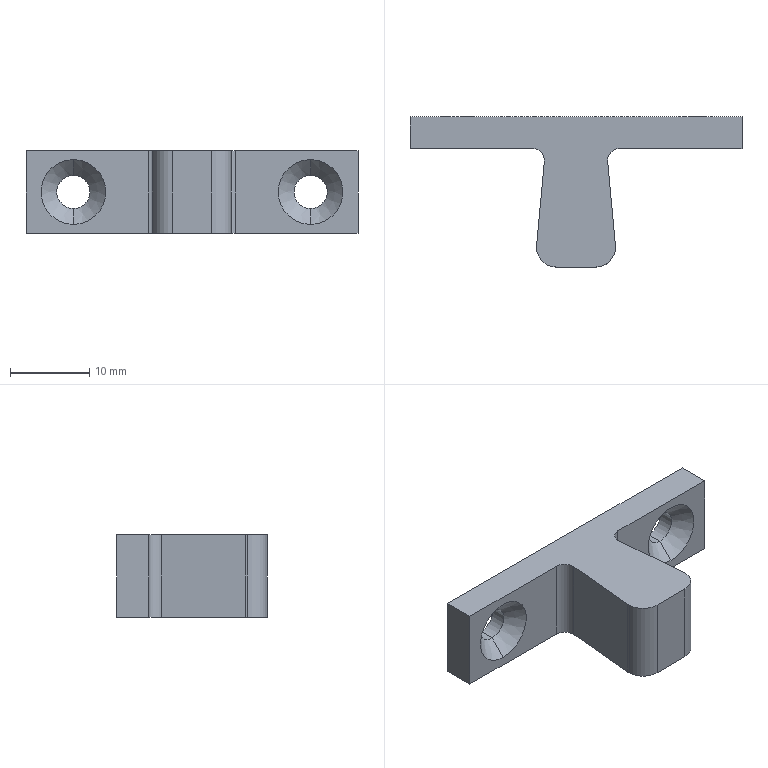Part | STEP file | CATCHE2_MISUMI_BCAS70_Latch | 1 solid | 24 faces | box 42 x 19 x 10.5 mm | volume 2994 mm3 | cylinder 10 | plane 10 | cone 4 | commonest cylinder face diameters 4.2 x4 3 x3 5 x3
STEP:
#1=CARTESIAN_POINT('',(-15.,-2.,2.1));
#2=VERTEX_POINT('',#1);
#3=CARTESIAN_POINT('',(-15.,-2.,-2.1));
#4=VERTEX_POINT('',#3);
#5=CARTESIAN_POINT('',(-15.,-2.,0.));
#6=DIRECTION('',(0.,-1.,0.));
#7=DIRECTION('',(0.,0.,-1.));
#8=AXIS2_PLACEMENT_3D('',#5,#6,#7);
#9=CIRCLE('',#8,2.1);
#10=EDGE_CURVE('',#2,#4,#9,.T.);
#11=ORIENTED_EDGE('',*,*,#10,.F.);
#12=CARTESIAN_POINT('',(-15.,-4.,4.1));
#13=VERTEX_POINT('',#12);
#14=CARTESIAN_POINT('',(-15.,-4.,4.1));
#15=DIRECTION('',(0.,-0.7071,0.7071));
#16=VECTOR('',#15,1000.);
#17=LINE('',#14,#16);
#18=EDGE_CURVE('',#2,#13,#17,.T.);
#19=ORIENTED_EDGE('',*,*,#18,.T.);
#20=CARTESIAN_POINT('',(-15.,-4.,-4.1));
#21=VERTEX_POINT('',#20);
#22=CARTESIAN_POINT('',(-15.,-4.,0.));
#23=DIRECTION('',(0.,-1.,0.));
#24=DIRECTION('',(0.,0.,-1.));
#25=AXIS2_PLACEMENT_3D('',#22,#23,#24);
#26=CIRCLE('',#25,4.1);
#27=EDGE_CURVE('',#13,#21,#26,.T.);
#28=ORIENTED_EDGE('',*,*,#27,.T.);
#29=CARTESIAN_POINT('',(-15.,-4.,-4.1));
#30=DIRECTION('',(0.,-0.7071,-0.7071));
#31=VECTOR('',#30,1000.);
#32=LINE('',#29,#31);
#33=EDGE_CURVE('',#4,#21,#32,.T.);
#34=ORIENTED_EDGE('',*,*,#33,.F.);
#35=EDGE_LOOP('',(#11,#19,#28,#34));
#36=FACE_OUTER_BOUND('',#35,.T.);
#37=CARTESIAN_POINT('',(-15.,-4.,0.));
#38=DIRECTION('',(0.,-1.,0.));
#39=DIRECTION('',(0.,0.,-1.));
#40=AXIS2_PLACEMENT_3D('',#37,#38,#39);
#41=CONICAL_SURFACE('',#40,4.1,0.7854);
#42=ADVANCED_FACE('',(#36),#41,.F.);
#43=CARTESIAN_POINT('',(-15.,0.,2.1));
#44=VERTEX_POINT('',#43);
#45=CARTESIAN_POINT('',(-15.,0.,-2.1));
#46=VERTEX_POINT('',#45);
#47=CARTESIAN_POINT('',(-15.,0.,0.));
#48=DIRECTION('',(0.,-1.,0.));
#49=DIRECTION('',(0.,0.,-1.));
#50=AXIS2_PLACEMENT_3D('',#47,#48,#49);
#51=CIRCLE('',#50,2.1);
#52=EDGE_CURVE('',#44,#46,#51,.T.);
#53=ORIENTED_EDGE('',*,*,#52,.F.);
#54=CARTESIAN_POINT('',(-15.,-4.,2.1));
#55=DIRECTION('',(0.,-1.,0.));
#56=VECTOR('',#55,1000.);
#57=LINE('',#54,#56);
#58=EDGE_CURVE('',#44,#2,#57,.T.);
#59=ORIENTED_EDGE('',*,*,#58,.T.);
#60=ORIENTED_EDGE('',*,*,#10,.T.);
#61=CARTESIAN_POINT('',(-15.,-4.,-2.1));
#62=DIRECTION('',(0.,-1.,0.));
#63=VECTOR('',#62,1000.);
#64=LINE('',#61,#63);
#65=EDGE_CURVE('',#46,#4,#64,.T.);
#66=ORIENTED_EDGE('',*,*,#65,.F.);
#67=EDGE_LOOP('',(#53,#59,#60,#66));
#68=FACE_OUTER_BOUND('',#67,.T.);
#69=CARTESIAN_POINT('',(-15.,-4.,0.));
#70=DIRECTION('',(0.,-1.,0.));
#71=DIRECTION('',(0.,0.,-1.));
#72=AXIS2_PLACEMENT_3D('',#69,#70,#71);
#73=CYLINDRICAL_SURFACE('',#72,2.1);
#74=ADVANCED_FACE('',(#68),#73,.F.);
#75=CARTESIAN_POINT('',(15.,-2.,2.1));
#76=VERTEX_POINT('',#75);
#77=CARTESIAN_POINT('',(15.,-2.,-2.1));
#78=VERTEX_POINT('',#77);
#79=CARTESIAN_POINT('',(15.,-2.,0.));
#80=DIRECTION('',(0.,-1.,0.));
#81=DIRECTION('',(0.,0.,-1.));
#82=AXIS2_PLACEMENT_3D('',#79,#80,#81);
#83=CIRCLE('',#82,2.1);
#84=EDGE_CURVE('',#76,#78,#83,.T.);
#85=ORIENTED_EDGE('',*,*,#84,.F.);
#86=CARTESIAN_POINT('',(15.,-4.,4.1));
#87=VERTEX_POINT('',#86);
#88=CARTESIAN_POINT('',(15.,-4.,4.1));
#89=DIRECTION('',(0.,-0.7071,0.7071));
#90=VECTOR('',#89,1000.);
#91=LINE('',#88,#90);
#92=EDGE_CURVE('',#76,#87,#91,.T.);
#93=ORIENTED_EDGE('',*,*,#92,.T.);
#94=CARTESIAN_POINT('',(15.,-4.,-4.1));
#95=VERTEX_POINT('',#94);
#96=CARTESIAN_POINT('',(15.,-4.,0.));
#97=DIRECTION('',(0.,-1.,0.));
#98=DIRECTION('',(0.,0.,-1.));
#99=AXIS2_PLACEMENT_3D('',#96,#97,#98);
#100=CIRCLE('',#99,4.1);
#101=EDGE_CURVE('',#87,#95,#100,.T.);
#102=ORIENTED_EDGE('',*,*,#101,.T.);
#103=CARTESIAN_POINT('',(15.,-4.,-4.1));
#104=DIRECTION('',(0.,-0.7071,-0.7071));
#105=VECTOR('',#104,1000.);
#106=LINE('',#103,#105);
#107=EDGE_CURVE('',#78,#95,#106,.T.);
#108=ORIENTED_EDGE('',*,*,#107,.F.);
#109=EDGE_LOOP('',(#85,#93,#102,#108));
#110=FACE_OUTER_BOUND('',#109,.T.);
#111=CARTESIAN_POINT('',(15.,-4.,0.));
#112=DIRECTION('',(0.,-1.,0.));
#113=DIRECTION('',(0.,0.,-1.));
#114=AXIS2_PLACEMENT_3D('',#111,#112,#113);
#115=CONICAL_SURFACE('',#114,4.1,0.7854);
#116=ADVANCED_FACE('',(#110),#115,.F.);
#117=CARTESIAN_POINT('',(15.,0.,2.1));
#118=VERTEX_POINT('',#117);
#119=CARTESIAN_POINT('',(15.,0.,-2.1));
#120=VERTEX_POINT('',#119);
#121=CARTESIAN_POINT('',(15.,0.,0.));
#122=DIRECTION('',(0.,-1.,0.));
#123=DIRECTION('',(0.,0.,-1.));
#124=AXIS2_PLACEMENT_3D('',#121,#122,#123);
#125=CIRCLE('',#124,2.1);
#126=EDGE_CURVE('',#118,#120,#125,.T.);
#127=ORIENTED_EDGE('',*,*,#126,.F.);
#128=CARTESIAN_POINT('',(15.,-4.,2.1));
#129=DIRECTION('',(0.,-1.,0.));
#130=VECTOR('',#129,1000.);
#131=LINE('',#128,#130);
#132=EDGE_CURVE('',#118,#76,#131,.T.);
#133=ORIENTED_EDGE('',*,*,#132,.T.);
#134=ORIENTED_EDGE('',*,*,#84,.T.);
#135=CARTESIAN_POINT('',(15.,-4.,-2.1));
#136=DIRECTION('',(0.,-1.,0.));
#137=VECTOR('',#136,1000.);
#138=LINE('',#135,#137);
#139=EDGE_CURVE('',#120,#78,#138,.T.);
#140=ORIENTED_EDGE('',*,*,#139,.F.);
#141=EDGE_LOOP('',(#127,#133,#134,#140));
#142=FACE_OUTER_BOUND('',#141,.T.);
#143=CARTESIAN_POINT('',(15.,-4.,0.));
#144=DIRECTION('',(0.,-1.,0.));
#145=DIRECTION('',(0.,0.,-1.));
#146=AXIS2_PLACEMENT_3D('',#143,#144,#145);
#147=CYLINDRICAL_SURFACE('',#146,2.1);
#148=ADVANCED_FACE('',(#142),#147,.F.);
#149=CARTESIAN_POINT('',(4.,-5.5,5.25));
#150=VERTEX_POINT('',#149);
#151=CARTESIAN_POINT('',(5.5,-4.,5.25));
#152=VERTEX_POINT('',#151);
#153=CARTESIAN_POINT('',(5.5,-5.5,5.25));
#154=DIRECTION('',(0.,0.,-1.));
#155=DIRECTION('',(1.,0.,0.));
#156=AXIS2_PLACEMENT_3D('',#153,#154,#155);
#157=CIRCLE('',#156,1.5);
#158=EDGE_CURVE('',#150,#152,#157,.T.);
#159=ORIENTED_EDGE('',*,*,#158,.F.);
#160=CARTESIAN_POINT('',(4.,-5.5,-5.25));
#161=VERTEX_POINT('',#160);
#162=CARTESIAN_POINT('',(4.,-5.5,5.25));
#163=DIRECTION('',(0.,0.,-1.));
#164=VECTOR('',#163,1000.);
#165=LINE('',#162,#164);
#166=EDGE_CURVE('',#150,#161,#165,.T.);
#167=ORIENTED_EDGE('',*,*,#166,.T.);
#168=CARTESIAN_POINT('',(5.5,-4.,-5.25));
#169=VERTEX_POINT('',#168);
#170=CARTESIAN_POINT('',(5.5,-5.5,-5.25));
#171=DIRECTION('',(0.,0.,-1.));
#172=DIRECTION('',(1.,0.,0.));
#173=AXIS2_PLACEMENT_3D('',#170,#171,#172);
#174=CIRCLE('',#173,1.5);
#175=EDGE_CURVE('',#161,#169,#174,.T.);
#176=ORIENTED_EDGE('',*,*,#175,.T.);
#177=CARTESIAN_POINT('',(5.5,-4.,5.25));
#178=DIRECTION('',(0.,0.,-1.));
#179=VECTOR('',#178,1000.);
#180=LINE('',#177,#179);
#181=EDGE_CURVE('',#152,#169,#180,.T.);
#182=ORIENTED_EDGE('',*,*,#181,.F.);
#183=EDGE_LOOP('',(#159,#167,#176,#182));
#184=FACE_OUTER_BOUND('',#183,.T.);
#185=CARTESIAN_POINT('',(5.5,-5.5,5.25));
#186=DIRECTION('',(0.,0.,-1.));
#187=DIRECTION('',(-1.,0.,0.));
#188=AXIS2_PLACEMENT_3D('',#185,#186,#187);
#189=CYLINDRICAL_SURFACE('',#188,1.5);
#190=ADVANCED_FACE('',(#184),#189,.F.);
#191=CARTESIAN_POINT('',(-5.,-16.5,5.25));
#192=VERTEX_POINT('',#191);
#193=CARTESIAN_POINT('',(-2.5,-19.,5.25));
#194=VERTEX_POINT('',#193);
#195=CARTESIAN_POINT('',(-2.5,-16.5,5.25));
#196=DIRECTION('',(0.,0.,1.));
#197=DIRECTION('',(1.,0.,0.));
#198=AXIS2_PLACEMENT_3D('',#195,#196,#197);
#199=CIRCLE('',#198,2.5);
#200=EDGE_CURVE('',#192,#194,#199,.T.);
#201=ORIENTED_EDGE('',*,*,#200,.F.);
#202=CARTESIAN_POINT('',(-5.,-16.5,-5.25));
#203=VERTEX_POINT('',#202);
#204=CARTESIAN_POINT('',(-5.,-16.5,5.25));
#205=DIRECTION('',(0.,0.,-1.));
#206=VECTOR('',#205,1000.);
#207=LINE('',#204,#206);
#208=EDGE_CURVE('',#192,#203,#207,.T.);
#209=ORIENTED_EDGE('',*,*,#208,.T.);
#210=CARTESIAN_POINT('',(-2.5,-19.,-5.25));
#211=VERTEX_POINT('',#210);
#212=CARTESIAN_POINT('',(-2.5,-16.5,-5.25));
#213=DIRECTION('',(0.,0.,1.));
#214=DIRECTION('',(1.,0.,0.));
#215=AXIS2_PLACEMENT_3D('',#212,#213,#214);
#216=CIRCLE('',#215,2.5);
#217=EDGE_CURVE('',#203,#211,#216,.T.);
#218=ORIENTED_EDGE('',*,*,#217,.T.);
#219=CARTESIAN_POINT('',(-2.5,-19.,5.25));
#220=DIRECTION('',(0.,0.,-1.));
#221=VECTOR('',#220,1000.);
#222=LINE('',#219,#221);
#223=EDGE_CURVE('',#194,#211,#222,.T.);
#224=ORIENTED_EDGE('',*,*,#223,.F.);
#225=EDGE_LOOP('',(#201,#209,#218,#224));
#226=FACE_OUTER_BOUND('',#225,.T.);
#227=CARTESIAN_POINT('',(-2.5,-16.5,5.25));
#228=DIRECTION('',(0.,0.,-1.));
#229=DIRECTION('',(-1.,0.,0.));
#230=AXIS2_PLACEMENT_3D('',#227,#228,#229);
#231=CYLINDRICAL_SURFACE('',#230,2.5);
#232=ADVANCED_FACE('',(#226),#231,.T.);
#233=CARTESIAN_POINT('',(21.,-4.,-5.25));
#234=VERTEX_POINT('',#233);
#235=CARTESIAN_POINT('',(21.,0.,-5.25));
#236=VERTEX_POINT('',#235);
#237=CARTESIAN_POINT('',(21.,-4.,-5.25));
#238=DIRECTION('',(0.,1.,0.));
#239=VECTOR('',#238,1000.);
#240=LINE('',#237,#239);
#241=EDGE_CURVE('',#234,#236,#240,.T.);
#242=ORIENTED_EDGE('',*,*,#241,.T.);
#243=CARTESIAN_POINT('',(21.,0.,5.25));
#244=VERTEX_POINT('',#243);
#245=CARTESIAN_POINT('',(21.,0.,5.25));
#246=DIRECTION('',(0.,0.,-1.));
#247=VECTOR('',#246,1000.);
#248=LINE('',#245,#247);
#249=EDGE_CURVE('',#244,#236,#248,.T.);
#250=ORIENTED_EDGE('',*,*,#249,.F.);
#251=CARTESIAN_POINT('',(21.,-4.,5.25));
#252=VERTEX_POINT('',#251);
#253=CARTESIAN_POINT('',(21.,-4.,5.25));
#254=DIRECTION('',(0.,1.,0.));
#255=VECTOR('',#254,1000.);
#256=LINE('',#253,#255);
#257=EDGE_CURVE('',#252,#244,#256,.T.);
#258=ORIENTED_EDGE('',*,*,#257,.F.);
#259=CARTESIAN_POINT('',(21.,-4.,5.25));
#260=DIRECTION('',(0.,0.,-1.));
#261=VECTOR('',#260,1000.);
#262=LINE('',#259,#261);
#263=EDGE_CURVE('',#252,#234,#262,.T.);
#264=ORIENTED_EDGE('',*,*,#263,.T.);
#265=EDGE_LOOP('',(#242,#250,#258,#264));
#266=FACE_OUTER_BOUND('',#265,.T.);
#267=CARTESIAN_POINT('',(21.,-4.,5.25));
#268=DIRECTION('',(-1.,0.,0.));
#269=DIRECTION('',(0.,0.,1.));
#270=AXIS2_PLACEMENT_3D('',#267,#268,#269);
#271=PLANE('',#270);
#272=ADVANCED_FACE('',(#266),#271,.F.);
#273=CARTESIAN_POINT('',(-15.,0.,0.));
#274=DIRECTION('',(0.,-1.,0.));
#275=DIRECTION('',(0.,0.,-1.));
#276=AXIS2_PLACEMENT_3D('',#273,#274,#275);
#277=CIRCLE('',#276,2.1);
#278=EDGE_CURVE('',#46,#44,#277,.T.);
#279=ORIENTED_EDGE('',*,*,#278,.T.);
#280=ORIENTED_EDGE('',*,*,#52,.T.);
#281=EDGE_LOOP('',(#279,#280));
#282=FACE_BOUND('',#281,.T.);
#283=CARTESIAN_POINT('',(15.,0.,0.));
#284=DIRECTION('',(0.,-1.,0.));
#285=DIRECTION('',(0.,0.,-1.));
#286=AXIS2_PLACEMENT_3D('',#283,#284,#285);
#287=CIRCLE('',#286,2.1);
#288=EDGE_CURVE('',#120,#118,#287,.T.);
#289=ORIENTED_EDGE('',*,*,#288,.T.);
#290=ORIENTED_EDGE('',*,*,#126,.T.);
#291=EDGE_LOOP('',(#289,#290));
#292=FACE_BOUND('',#291,.T.);
#293=CARTESIAN_POINT('',(-21.,0.,-5.25));
#294=VERTEX_POINT('',#293);
#295=CARTESIAN_POINT('',(21.,0.,-5.25));
#296=DIRECTION('',(-1.,0.,0.));
#297=VECTOR('',#296,1000.);
#298=LINE('',#295,#297);
#299=EDGE_CURVE('',#236,#294,#298,.T.);
#300=ORIENTED_EDGE('',*,*,#299,.T.);
#301=CARTESIAN_POINT('',(-21.,0.,5.25));
#302=VERTEX_POINT('',#301);
#303=CARTESIAN_POINT('',(-21.,0.,5.25));
#304=DIRECTION('',(0.,0.,-1.));
#305=VECTOR('',#304,1000.);
#306=LINE('',#303,#305);
#307=EDGE_CURVE('',#302,#294,#306,.T.);
#308=ORIENTED_EDGE('',*,*,#307,.F.);
#309=CARTESIAN_POINT('',(21.,0.,5.25));
#310=DIRECTION('',(-1.,0.,0.));
#311=VECTOR('',#310,1000.);
#312=LINE('',#309,#311);
#313=EDGE_CURVE('',#244,#302,#312,.T.);
#314=ORIENTED_EDGE('',*,*,#313,.F.);
#315=ORIENTED_EDGE('',*,*,#249,.T.);
#316=EDGE_LOOP('',(#300,#308,#314,#315));
#317=FACE_OUTER_BOUND('',#316,.T.);
#318=CARTESIAN_POINT('',(21.,0.,5.25));
#319=DIRECTION('',(0.,-1.,0.));
#320=DIRECTION('',(1.,0.,0.));
#321=AXIS2_PLACEMENT_3D('',#318,#319,#320);
#322=PLANE('',#321);
#323=ADVANCED_FACE('',(#282,#292,#317),#322,.F.);
#324=CARTESIAN_POINT('',(-21.,-4.,-5.25));
#325=VERTEX_POINT('',#324);
#326=CARTESIAN_POINT('',(-21.,-4.,-5.25));
#327=DIRECTION('',(0.,-1.,0.));
#328=VECTOR('',#327,1000.);
#329=LINE('',#326,#328);
#330=EDGE_CURVE('',#294,#325,#329,.T.);
#331=ORIENTED_EDGE('',*,*,#330,.T.);
#332=CARTESIAN_POINT('',(-21.,-4.,5.25));
#333=VERTEX_POINT('',#332);
#334=CARTESIAN_POINT('',(-21.,-4.,5.25));
#335=DIRECTION('',(0.,0.,-1.));
#336=VECTOR('',#335,1000.);
#337=LINE('',#334,#336);
#338=EDGE_CURVE('',#333,#325,#337,.T.);
#339=ORIENTED_EDGE('',*,*,#338,.F.);
#340=CARTESIAN_POINT('',(-21.,-4.,5.25));
#341=DIRECTION('',(0.,-1.,0.));
#342=VECTOR('',#341,1000.);
#343=LINE('',#340,#342);
#344=EDGE_CURVE('',#302,#333,#343,.T.);
#345=ORIENTED_EDGE('',*,*,#344,.F.);
#346=ORIENTED_EDGE('',*,*,#307,.T.);
#347=EDGE_LOOP('',(#331,#339,#345,#346));
#348=FACE_OUTER_BOUND('',#347,.T.);
#349=CARTESIAN_POINT('',(-21.,-4.,5.25));
#350=DIRECTION('',(1.,0.,0.));
#351=DIRECTION('',(0.,0.,-1.));
#352=AXIS2_PLACEMENT_3D('',#349,#350,#351);
#353=PLANE('',#352);
#354=ADVANCED_FACE('',(#348),#353,.F.);
#355=CARTESIAN_POINT('',(-15.,-4.,0.));
#356=DIRECTION('',(0.,-1.,0.));
#357=DIRECTION('',(0.,0.,-1.));
#358=AXIS2_PLACEMENT_3D('',#355,#356,#357);
#359=CIRCLE('',#358,4.1);
#360=EDGE_CURVE('',#21,#13,#359,.T.);
#361=ORIENTED_EDGE('',*,*,#360,.F.);
#362=ORIENTED_EDGE('',*,*,#27,.F.);
#363=EDGE_LOOP('',(#361,#362));
#364=FACE_BOUND('',#363,.T.);
#365=CARTESIAN_POINT('',(-5.5,-4.,-5.25));
#366=VERTEX_POINT('',#365);
#367=CARTESIAN_POINT('',(-21.,-4.,-5.25));
#368=DIRECTION('',(1.,0.,0.));
#369=VECTOR('',#368,1000.);
#370=LINE('',#367,#369);
#371=EDGE_CURVE('',#325,#366,#370,.T.);
#372=ORIENTED_EDGE('',*,*,#371,.T.);
#373=CARTESIAN_POINT('',(-5.5,-4.,5.25));
#374=VERTEX_POINT('',#373);
#375=CARTESIAN_POINT('',(-5.5,-4.,5.25));
#376=DIRECTION('',(0.,0.,-1.));
#377=VECTOR('',#376,1000.);
#378=LINE('',#375,#377);
#379=EDGE_CURVE('',#374,#366,#378,.T.);
#380=ORIENTED_EDGE('',*,*,#379,.F.);
#381=CARTESIAN_POINT('',(-21.,-4.,5.25));
#382=DIRECTION('',(1.,0.,0.));
#383=VECTOR('',#382,1000.);
#384=LINE('',#381,#383);
#385=EDGE_CURVE('',#333,#374,#384,.T.);
#386=ORIENTED_EDGE('',*,*,#385,.F.);
#387=ORIENTED_EDGE('',*,*,#338,.T.);
#388=EDGE_LOOP('',(#372,#380,#386,#387));
#389=FACE_OUTER_BOUND('',#388,.T.);
#390=CARTESIAN_POINT('',(-21.,-4.,5.25));
#391=DIRECTION('',(0.,1.,0.));
#392=DIRECTION('',(-1.,0.,0.));
#393=AXIS2_PLACEMENT_3D('',#390,#391,#392);
#394=PLANE('',#393);
#395=ADVANCED_FACE('',(#364,#389),#394,.F.);
#396=CARTESIAN_POINT('',(-4.006,-5.638,-5.25));
#397=VERTEX_POINT('',#396);
#398=CARTESIAN_POINT('',(-5.5,-5.5,-5.25));
#399=DIRECTION('',(0.,0.,-1.));
#400=DIRECTION('',(-1.,0.,0.));
#401=AXIS2_PLACEMENT_3D('',#398,#399,#400);
#402=CIRCLE('',#401,1.5);
#403=EDGE_CURVE('',#366,#397,#402,.T.);
#404=ORIENTED_EDGE('',*,*,#403,.T.);
#405=CARTESIAN_POINT('',(-4.006,-5.638,5.25));
#406=VERTEX_POINT('',#405);
#407=CARTESIAN_POINT('',(-4.006,-5.638,5.25));
#408=DIRECTION('',(0.,0.,-1.));
#409=VECTOR('',#408,1000.);
#410=LINE('',#407,#409);
#411=EDGE_CURVE('',#406,#397,#410,.T.);
#412=ORIENTED_EDGE('',*,*,#411,.F.);
#413=CARTESIAN_POINT('',(-5.5,-5.5,5.25));
#414=DIRECTION('',(0.,0.,-1.));
#415=DIRECTION('',(-1.,0.,0.));
#416=AXIS2_PLACEMENT_3D('',#413,#414,#415);
#417=CIRCLE('',#416,1.5);
#418=EDGE_CURVE('',#374,#406,#417,.T.);
#419=ORIENTED_EDGE('',*,*,#418,.F.);
#420=ORIENTED_EDGE('',*,*,#379,.T.);
#421=EDGE_LOOP('',(#404,#412,#419,#420));
#422=FACE_OUTER_BOUND('',#421,.T.);
#423=CARTESIAN_POINT('',(-5.5,-5.5,5.25));
#424=DIRECTION('',(0.,0.,-1.));
#425=DIRECTION('',(-1.,0.,0.));
#426=AXIS2_PLACEMENT_3D('',#423,#424,#425);
#427=CYLINDRICAL_SURFACE('',#426,1.5);
#428=ADVANCED_FACE('',(#422),#427,.F.);
#429=CARTESIAN_POINT('',(-4.989,-16.27,-5.25));
#430=VERTEX_POINT('',#429);
#431=CARTESIAN_POINT('',(-4.006,-5.638,-5.25));
#432=DIRECTION('',(-0.09207,-0.9958,0.));
#433=VECTOR('',#432,1000.);
#434=LINE('',#431,#433);
#435=EDGE_CURVE('',#397,#430,#434,.T.);
#436=ORIENTED_EDGE('',*,*,#435,.T.);
#437=CARTESIAN_POINT('',(-4.989,-16.27,5.25));
#438=VERTEX_POINT('',#437);
#439=CARTESIAN_POINT('',(-4.989,-16.27,5.25));
#440=DIRECTION('',(0.,0.,-1.));
#441=VECTOR('',#440,1000.);
#442=LINE('',#439,#441);
#443=EDGE_CURVE('',#438,#430,#442,.T.);
#444=ORIENTED_EDGE('',*,*,#443,.F.);
#445=CARTESIAN_POINT('',(-4.006,-5.638,5.25));
#446=DIRECTION('',(-0.09207,-0.9958,0.));
#447=VECTOR('',#446,1000.);
#448=LINE('',#445,#447);
#449=EDGE_CURVE('',#406,#438,#448,.T.);
#450=ORIENTED_EDGE('',*,*,#449,.F.);
#451=ORIENTED_EDGE('',*,*,#411,.T.);
#452=EDGE_LOOP('',(#436,#444,#450,#451));
#453=FACE_OUTER_BOUND('',#452,.T.);
#454=CARTESIAN_POINT('',(-4.006,-5.638,5.25));
#455=DIRECTION('',(0.9958,-0.09207,0.));
#456=DIRECTION('',(0.09207,0.9958,0.));
#457=AXIS2_PLACEMENT_3D('',#454,#455,#456);
#458=PLANE('',#457);
#459=ADVANCED_FACE('',(#453),#458,.F.);
#460=ORIENTED_EDGE('',*,*,#208,.F.);
#461=CARTESIAN_POINT('',(-2.5,-16.5,5.25));
#462=DIRECTION('',(0.,0.,1.));
#463=DIRECTION('',(1.,0.,0.));
#464=AXIS2_PLACEMENT_3D('',#461,#462,#463);
#465=CIRCLE('',#464,2.5);
#466=EDGE_CURVE('',#438,#192,#465,.T.);
#467=ORIENTED_EDGE('',*,*,#466,.F.);
#468=ORIENTED_EDGE('',*,*,#443,.T.);
#469=CARTESIAN_POINT('',(-2.5,-16.5,-5.25));
#470=DIRECTION('',(0.,0.,1.));
#471=DIRECTION('',(1.,0.,0.));
#472=AXIS2_PLACEMENT_3D('',#469,#470,#471);
#473=CIRCLE('',#472,2.5);
#474=EDGE_CURVE('',#430,#203,#473,.T.);
#475=ORIENTED_EDGE('',*,*,#474,.T.);
#476=EDGE_LOOP('',(#460,#467,#468,#475));
#477=FACE_OUTER_BOUND('',#476,.T.);
#478=CARTESIAN_POINT('',(-2.5,-16.5,5.25));
#479=DIRECTION('',(0.,0.,-1.));
#480=DIRECTION('',(-1.,0.,0.));
#481=AXIS2_PLACEMENT_3D('',#478,#479,#480);
#482=CYLINDRICAL_SURFACE('',#481,2.5);
#483=ADVANCED_FACE('',(#477),#482,.T.);
#484=CARTESIAN_POINT('',(2.5,-19.,-5.25));
#485=VERTEX_POINT('',#484);
#486=CARTESIAN_POINT('',(-2.5,-19.,-5.25));
#487=DIRECTION('',(1.,0.,0.));
#488=VECTOR('',#487,1000.);
#489=LINE('',#486,#488);
#490=EDGE_CURVE('',#211,#485,#489,.T.);
#491=ORIENTED_EDGE('',*,*,#490,.T.);
#492=CARTESIAN_POINT('',(2.5,-19.,5.25));
#493=VERTEX_POINT('',#492);
#494=CARTESIAN_POINT('',(2.5,-19.,5.25));
#495=DIRECTION('',(0.,0.,-1.));
#496=VECTOR('',#495,1000.);
#497=LINE('',#494,#496);
#498=EDGE_CURVE('',#493,#485,#497,.T.);
#499=ORIENTED_EDGE('',*,*,#498,.F.);
#500=CARTESIAN_POINT('',(-2.5,-19.,5.25));
#501=DIRECTION('',(1.,0.,0.));
#502=VECTOR('',#501,1000.);
#503=LINE('',#500,#502);
#504=EDGE_CURVE('',#194,#493,#503,.T.);
#505=ORIENTED_EDGE('',*,*,#504,.F.);
#506=ORIENTED_EDGE('',*,*,#223,.T.);
#507=EDGE_LOOP('',(#491,#499,#505,#506));
#508=FACE_OUTER_BOUND('',#507,.T.);
#509=CARTESIAN_POINT('',(-2.5,-19.,5.25));
#510=DIRECTION('',(0.,1.,0.));
#511=DIRECTION('',(0.,0.,1.));
#512=AXIS2_PLACEMENT_3D('',#509,#510,#511);
#513=PLANE('',#512);
#514=ADVANCED_FACE('',(#508),#513,.F.);
#515=CARTESIAN_POINT('',(4.989,-16.27,-5.25));
#516=VERTEX_POINT('',#515);
#517=CARTESIAN_POINT('',(2.5,-16.5,-5.25));
#518=DIRECTION('',(0.,0.,1.));
#519=DIRECTION('',(-1.,0.,0.));
#520=AXIS2_PLACEMENT_3D('',#517,#518,#519);
#521=CIRCLE('',#520,2.5);
#522=EDGE_CURVE('',#485,#516,#521,.T.);
#523=ORIENTED_EDGE('',*,*,#522,.T.);
#524=CARTESIAN_POINT('',(4.989,-16.27,5.25));
#525=VERTEX_POINT('',#524);
#526=CARTESIAN_POINT('',(4.989,-16.27,5.25));
#527=DIRECTION('',(0.,0.,-1.));
#528=VECTOR('',#527,1000.);
#529=LINE('',#526,#528);
#530=EDGE_CURVE('',#525,#516,#529,.T.);
#531=ORIENTED_EDGE('',*,*,#530,.F.);
#532=CARTESIAN_POINT('',(2.5,-16.5,5.25));
#533=DIRECTION('',(0.,0.,1.));
#534=DIRECTION('',(-1.,0.,0.));
#535=AXIS2_PLACEMENT_3D('',#532,#533,#534);
#536=CIRCLE('',#535,2.5);
#537=EDGE_CURVE('',#493,#525,#536,.T.);
#538=ORIENTED_EDGE('',*,*,#537,.F.);
#539=ORIENTED_EDGE('',*,*,#498,.T.);
#540=EDGE_LOOP('',(#523,#531,#538,#539));
#541=FACE_OUTER_BOUND('',#540,.T.);
#542=CARTESIAN_POINT('',(2.5,-16.5,5.25));
#543=DIRECTION('',(0.,0.,-1.));
#544=DIRECTION('',(-1.,0.,0.));
#545=AXIS2_PLACEMENT_3D('',#542,#543,#544);
#546=CYLINDRICAL_SURFACE('',#545,2.5);
#547=ADVANCED_FACE('',(#541),#546,.T.);
#548=CARTESIAN_POINT('',(4.006,-5.638,-5.25));
#549=VERTEX_POINT('',#548);
#550=CARTESIAN_POINT('',(4.006,-5.638,-5.25));
#551=DIRECTION('',(-0.09207,0.9958,0.));
#552=VECTOR('',#551,1000.);
#553=LINE('',#550,#552);
#554=EDGE_CURVE('',#516,#549,#553,.T.);
#555=ORIENTED_EDGE('',*,*,#554,.T.);
#556=CARTESIAN_POINT('',(4.006,-5.638,5.25));
#557=VERTEX_POINT('',#556);
#558=CARTESIAN_POINT('',(4.006,-5.638,5.25));
#559=DIRECTION('',(0.,0.,-1.));
#560=VECTOR('',#559,1000.);
#561=LINE('',#558,#560);
#562=EDGE_CURVE('',#557,#549,#561,.T.);
#563=ORIENTED_EDGE('',*,*,#562,.F.);
#564=CARTESIAN_POINT('',(4.006,-5.638,5.25));
#565=DIRECTION('',(-0.09207,0.9958,0.));
#566=VECTOR('',#565,1000.);
#567=LINE('',#564,#566);
#568=EDGE_CURVE('',#525,#557,#567,.T.);
#569=ORIENTED_EDGE('',*,*,#568,.F.);
#570=ORIENTED_EDGE('',*,*,#530,.T.);
#571=EDGE_LOOP('',(#555,#563,#569,#570));
#572=FACE_OUTER_BOUND('',#571,.T.);
#573=CARTESIAN_POINT('',(4.006,-5.638,5.25));
#574=DIRECTION('',(-0.9958,-0.09207,0.));
#575=DIRECTION('',(0.09207,-0.9958,0.));
#576=AXIS2_PLACEMENT_3D('',#573,#574,#575);
#577=PLANE('',#576);
#578=ADVANCED_FACE('',(#572),#577,.F.);
#579=ORIENTED_EDGE('',*,*,#166,.F.);
#580=CARTESIAN_POINT('',(5.5,-5.5,5.25));
#581=DIRECTION('',(0.,0.,-1.));
#582=DIRECTION('',(1.,0.,0.));
#583=AXIS2_PLACEMENT_3D('',#580,#581,#582);
#584=CIRCLE('',#583,1.5);
#585=EDGE_CURVE('',#557,#150,#584,.T.);
#586=ORIENTED_EDGE('',*,*,#585,.F.);
#587=ORIENTED_EDGE('',*,*,#562,.T.);
#588=CARTESIAN_POINT('',(5.5,-5.5,-5.25));
#589=DIRECTION('',(0.,0.,-1.));
#590=DIRECTION('',(1.,0.,0.));
#591=AXIS2_PLACEMENT_3D('',#588,#589,#590);
#592=CIRCLE('',#591,1.5);
#593=EDGE_CURVE('',#549,#161,#592,.T.);
#594=ORIENTED_EDGE('',*,*,#593,.T.);
#595=EDGE_LOOP('',(#579,#586,#587,#594));
#596=FACE_OUTER_BOUND('',#595,.T.);
#597=CARTESIAN_POINT('',(5.5,-5.5,5.25));
#598=DIRECTION('',(0.,0.,-1.));
#599=DIRECTION('',(-1.,0.,0.));
#600=AXIS2_PLACEMENT_3D('',#597,#598,#599);
#601=CYLINDRICAL_SURFACE('',#600,1.5);
#602=ADVANCED_FACE('',(#596),#601,.F.);
#603=CARTESIAN_POINT('',(15.,-4.,0.));
#604=DIRECTION('',(0.,-1.,0.));
#605=DIRECTION('',(0.,0.,-1.));
#606=AXIS2_PLACEMENT_3D('',#603,#604,#605);
#607=CIRCLE('',#606,4.1);
#608=EDGE_CURVE('',#95,#87,#607,.T.);
#609=ORIENTED_EDGE('',*,*,#608,.F.);
#610=ORIENTED_EDGE('',*,*,#101,.F.);
#611=EDGE_LOOP('',(#609,#610));
#612=FACE_BOUND('',#611,.T.);
#613=CARTESIAN_POINT('',(21.,-4.,-5.25));
#614=DIRECTION('',(1.,0.,0.));
#615=VECTOR('',#614,1000.);
#616=LINE('',#613,#615);
#617=EDGE_CURVE('',#169,#234,#616,.T.);
#618=ORIENTED_EDGE('',*,*,#617,.T.);
#619=ORIENTED_EDGE('',*,*,#263,.F.);
#620=CARTESIAN_POINT('',(21.,-4.,5.25));
#621=DIRECTION('',(1.,0.,0.));
#622=VECTOR('',#621,1000.);
#623=LINE('',#620,#622);
#624=EDGE_CURVE('',#152,#252,#623,.T.);
#625=ORIENTED_EDGE('',*,*,#624,.F.);
#626=ORIENTED_EDGE('',*,*,#181,.T.);
#627=EDGE_LOOP('',(#618,#619,#625,#626));
#628=FACE_OUTER_BOUND('',#627,.T.);
#629=CARTESIAN_POINT('',(21.,-4.,5.25));
#630=DIRECTION('',(0.,1.,0.));
#631=DIRECTION('',(0.,0.,1.));
#632=AXIS2_PLACEMENT_3D('',#629,#630,#631);
#633=PLANE('',#632);
#634=ADVANCED_FACE('',(#612,#628),#633,.F.);
#635=ORIENTED_EDGE('',*,*,#257,.T.);
#636=ORIENTED_EDGE('',*,*,#313,.T.);
#637=ORIENTED_EDGE('',*,*,#344,.T.);
#638=ORIENTED_EDGE('',*,*,#385,.T.);
#639=ORIENTED_EDGE('',*,*,#418,.T.);
#640=ORIENTED_EDGE('',*,*,#449,.T.);
#641=ORIENTED_EDGE('',*,*,#466,.T.);
#642=ORIENTED_EDGE('',*,*,#200,.T.);
#643=ORIENTED_EDGE('',*,*,#504,.T.);
#644=ORIENTED_EDGE('',*,*,#537,.T.);
#645=ORIENTED_EDGE('',*,*,#568,.T.);
#646=ORIENTED_EDGE('',*,*,#585,.T.);
#647=ORIENTED_EDGE('',*,*,#158,.T.);
#648=ORIENTED_EDGE('',*,*,#624,.T.);
#649=EDGE_LOOP('',(#635,#636,#637,#638,#639,#640,#641,#642,#643,#644,#645,#646,#647,#648));
#650=FACE_OUTER_BOUND('',#649,.T.);
#651=CARTESIAN_POINT('',(-5.5,-5.5,5.25));
#652=DIRECTION('',(0.,0.,-1.));
#653=DIRECTION('',(-1.,0.,0.));
#654=AXIS2_PLACEMENT_3D('',#651,#652,#653);
#655=PLANE('',#654);
#656=ADVANCED_FACE('',(#650),#655,.F.);
#657=ORIENTED_EDGE('',*,*,#241,.F.);
#658=ORIENTED_EDGE('',*,*,#617,.F.);
#659=ORIENTED_EDGE('',*,*,#175,.F.);
#660=ORIENTED_EDGE('',*,*,#593,.F.);
#661=ORIENTED_EDGE('',*,*,#554,.F.);
#662=ORIENTED_EDGE('',*,*,#522,.F.);
#663=ORIENTED_EDGE('',*,*,#490,.F.);
#664=ORIENTED_EDGE('',*,*,#217,.F.);
#665=ORIENTED_EDGE('',*,*,#474,.F.);
#666=ORIENTED_EDGE('',*,*,#435,.F.);
#667=ORIENTED_EDGE('',*,*,#403,.F.);
#668=ORIENTED_EDGE('',*,*,#371,.F.);
#669=ORIENTED_EDGE('',*,*,#330,.F.);
#670=ORIENTED_EDGE('',*,*,#299,.F.);
#671=EDGE_LOOP('',(#657,#658,#659,#660,#661,#662,#663,#664,#665,#666,#667,#668,#669,#670));
#672=FACE_OUTER_BOUND('',#671,.T.);
#673=CARTESIAN_POINT('',(-5.5,-5.5,-5.25));
#674=DIRECTION('',(0.,0.,-1.));
#675=DIRECTION('',(-1.,0.,0.));
#676=AXIS2_PLACEMENT_3D('',#673,#674,#675);
#677=PLANE('',#676);
#678=ADVANCED_FACE('',(#672),#677,.T.);
#679=ORIENTED_EDGE('',*,*,#132,.F.);
#680=ORIENTED_EDGE('',*,*,#288,.F.);
#681=ORIENTED_EDGE('',*,*,#139,.T.);
#682=CARTESIAN_POINT('',(15.,-2.,0.));
#683=DIRECTION('',(0.,-1.,0.));
#684=DIRECTION('',(0.,0.,-1.));
#685=AXIS2_PLACEMENT_3D('',#682,#683,#684);
#686=CIRCLE('',#685,2.1);
#687=EDGE_CURVE('',#78,#76,#686,.T.);
#688=ORIENTED_EDGE('',*,*,#687,.T.);
#689=EDGE_LOOP('',(#679,#680,#681,#688));
#690=FACE_OUTER_BOUND('',#689,.T.);
#691=CARTESIAN_POINT('',(15.,-4.,0.));
#692=DIRECTION('',(0.,-1.,0.));
#693=DIRECTION('',(0.,0.,-1.));
#694=AXIS2_PLACEMENT_3D('',#691,#692,#693);
#695=CYLINDRICAL_SURFACE('',#694,2.1);
#696=ADVANCED_FACE('',(#690),#695,.F.);
#697=ORIENTED_EDGE('',*,*,#92,.F.);
#698=ORIENTED_EDGE('',*,*,#687,.F.);
#699=ORIENTED_EDGE('',*,*,#107,.T.);
#700=ORIENTED_EDGE('',*,*,#608,.T.);
#701=EDGE_LOOP('',(#697,#698,#699,#700));
#702=FACE_OUTER_BOUND('',#701,.T.);
#703=CARTESIAN_POINT('',(15.,-4.,0.));
#704=DIRECTION('',(0.,-1.,0.));
#705=DIRECTION('',(0.,0.,-1.));
#706=AXIS2_PLACEMENT_3D('',#703,#704,#705);
#707=CONICAL_SURFACE('',#706,4.1,0.7854);
#708=ADVANCED_FACE('',(#702),#707,.F.);
#709=ORIENTED_EDGE('',*,*,#58,.F.);
#710=ORIENTED_EDGE('',*,*,#278,.F.);
#711=ORIENTED_EDGE('',*,*,#65,.T.);
#712=CARTESIAN_POINT('',(-15.,-2.,0.));
#713=DIRECTION('',(0.,-1.,0.));
#714=DIRECTION('',(0.,0.,-1.));
#715=AXIS2_PLACEMENT_3D('',#712,#713,#714);
#716=CIRCLE('',#715,2.1);
#717=EDGE_CURVE('',#4,#2,#716,.T.);
#718=ORIENTED_EDGE('',*,*,#717,.T.);
#719=EDGE_LOOP('',(#709,#710,#711,#718));
#720=FACE_OUTER_BOUND('',#719,.T.);
#721=CARTESIAN_POINT('',(-15.,-4.,0.));
#722=DIRECTION('',(0.,-1.,0.));
#723=DIRECTION('',(0.,0.,-1.));
#724=AXIS2_PLACEMENT_3D('',#721,#722,#723);
#725=CYLINDRICAL_SURFACE('',#724,2.1);
#726=ADVANCED_FACE('',(#720),#725,.F.);
#727=ORIENTED_EDGE('',*,*,#18,.F.);
#728=ORIENTED_EDGE('',*,*,#717,.F.);
#729=ORIENTED_EDGE('',*,*,#33,.T.);
#730=ORIENTED_EDGE('',*,*,#360,.T.);
#731=EDGE_LOOP('',(#727,#728,#729,#730));
#732=FACE_OUTER_BOUND('',#731,.T.);
#733=CARTESIAN_POINT('',(-15.,-4.,0.));
#734=DIRECTION('',(0.,-1.,0.));
#735=DIRECTION('',(0.,0.,-1.));
#736=AXIS2_PLACEMENT_3D('',#733,#734,#735);
#737=CONICAL_SURFACE('',#736,4.1,0.7854);
#738=ADVANCED_FACE('',(#732),#737,.F.);
#739=CLOSED_SHELL('',(#42,#74,#116,#148,#190,#232,#272,#323,#354,#395,#428,#459,#483,#514,#547,#578,#602,#634,#656,#678,#696,#708,#726,#738));
#740=MANIFOLD_SOLID_BREP('',#739);
#741=CARTESIAN_POINT('',(0.,0.,0.));
#742=DIRECTION('',(0.,0.,1.));
#743=DIRECTION('',(1.,0.,0.));
#744=AXIS2_PLACEMENT_3D('',#741,#742,#743);
#745=(LENGTH_UNIT()NAMED_UNIT(*)SI_UNIT(.MILLI.,.METRE.));
#746=UNCERTAINTY_MEASURE_WITH_UNIT(LENGTH_MEASURE(0.00001),#745,'','');
#747=(NAMED_UNIT(*)PLANE_ANGLE_UNIT()SI_UNIT($,.RADIAN.));
#748=(NAMED_UNIT(*)SI_UNIT($,.STERADIAN.)SOLID_ANGLE_UNIT());
#749=(GEOMETRIC_REPRESENTATION_CONTEXT(3)GLOBAL_UNCERTAINTY_ASSIGNED_CONTEXT((#746))GLOBAL_UNIT_ASSIGNED_CONTEXT((#745,#747,#748))REPRESENTATION_CONTEXT('',''));
#750=ADVANCED_BREP_SHAPE_REPRESENTATION('',(#740,#744),#749);